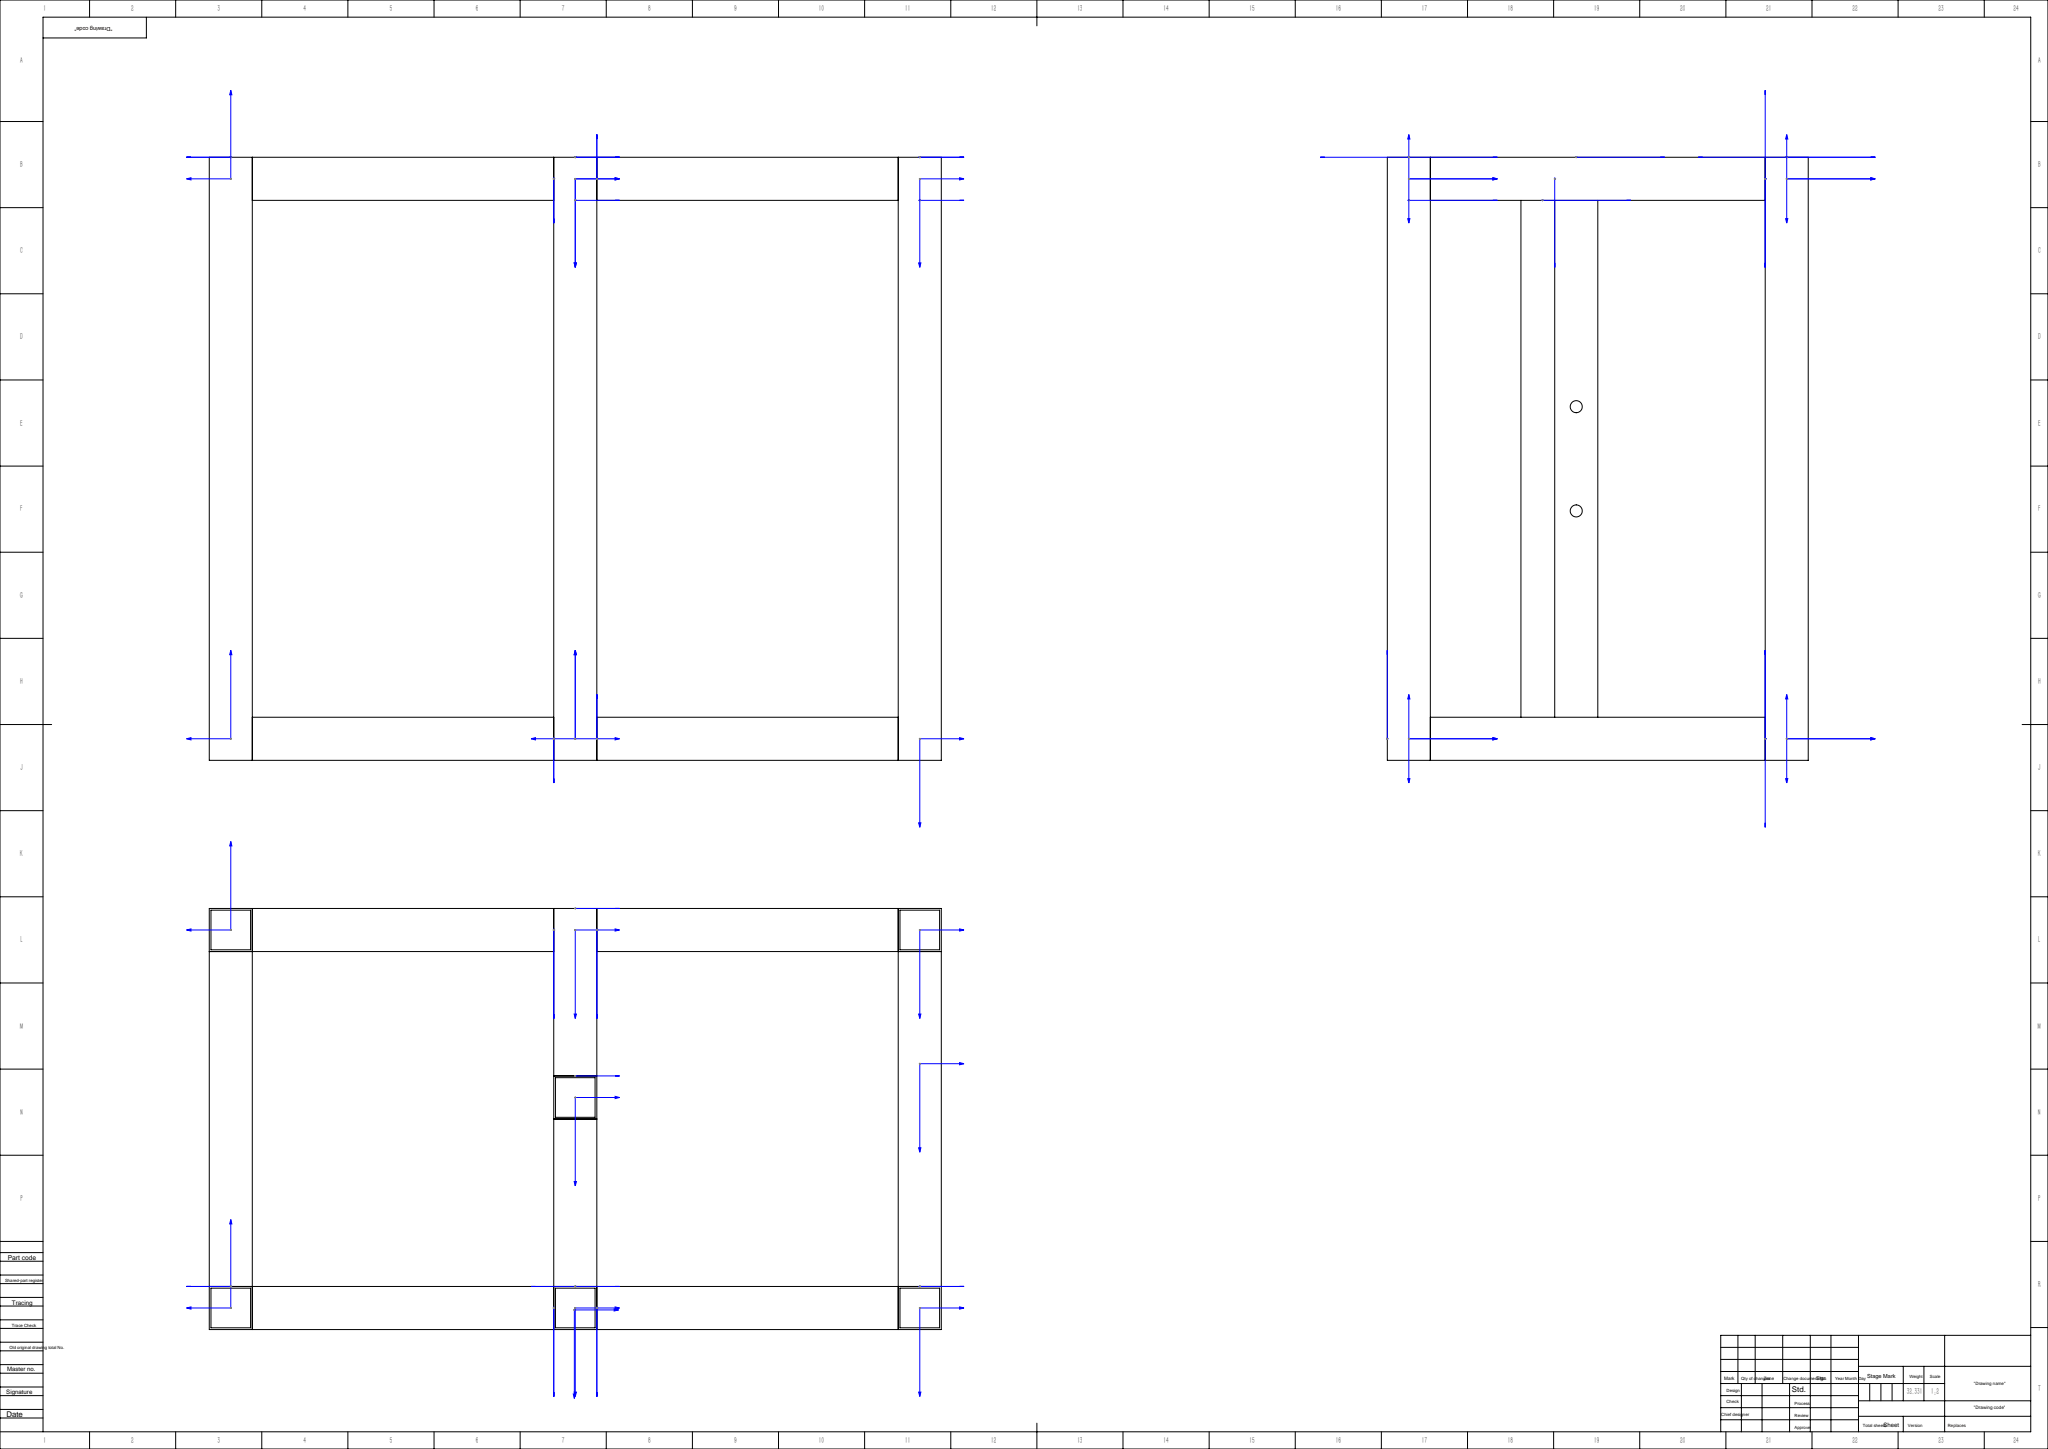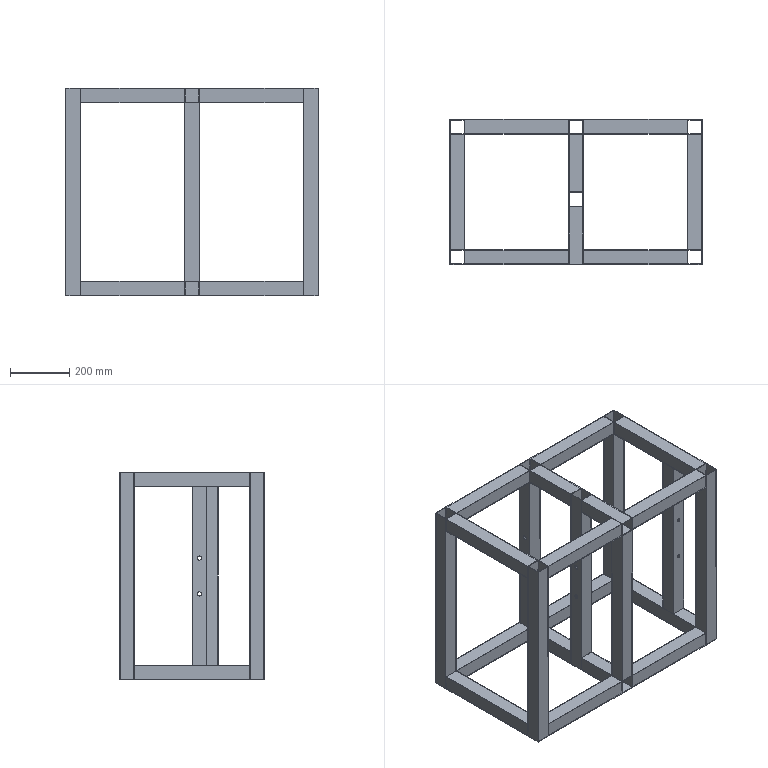Part | SolidWorks | 24 solids | 264 faces | box 850 x 488.8 x 700 mm | volume 4041372 mm3 | plane 240 | cylinder 24 | commonest cylinder face diameters 14 x16 11 x8